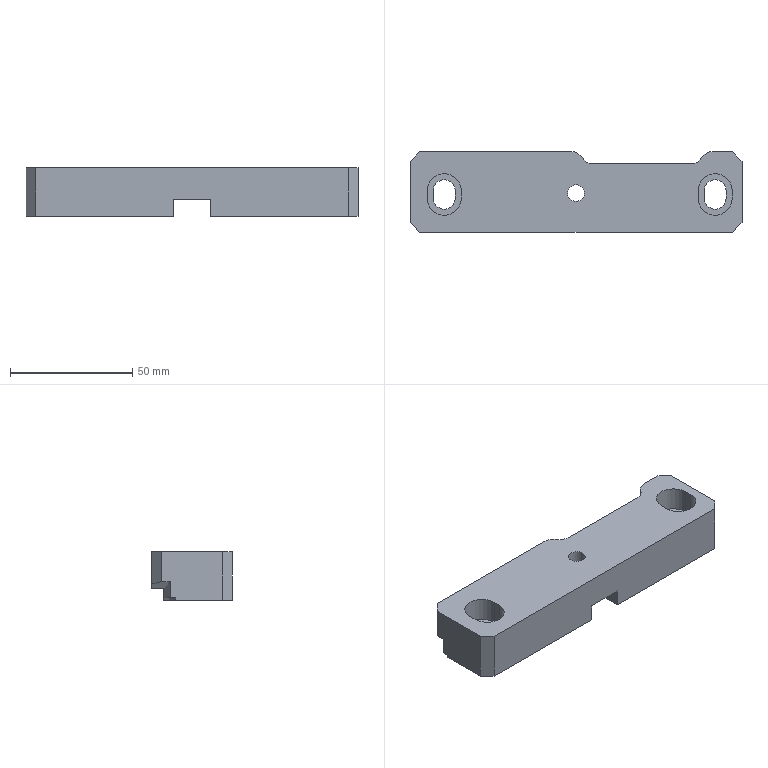Part | NX | features 20 2 | 1 solid | 49 faces | box 136 x 33 x 20 mm | volume 72364 mm3 | plane 35 | cylinder 14 | commonest cylinder face diameters 9 x4 10 x4 14 x4 6.8 x1 24 x1
STEP:
#1=CARTESIAN_POINT('',(810.268,-417.5,16.5));
#2=VERTEX_POINT('',#1);
#3=CARTESIAN_POINT('',(748.002,-417.5,16.5));
#4=VERTEX_POINT('',#3);
#5=CARTESIAN_POINT('',(932.002,-417.5,16.5));
#6=DIRECTION('',(-1.,0.,0.));
#7=VECTOR('',#6,1000.);
#8=LINE('',#5,#7);
#9=EDGE_CURVE('',#2,#4,#8,.T.);
#10=ORIENTED_EDGE('',*,*,#9,.T.);
#11=CARTESIAN_POINT('',(744.002,-421.5,16.5));
#12=VERTEX_POINT('',#11);
#13=CARTESIAN_POINT('',(744.002,-421.5,16.5));
#14=DIRECTION('',(-0.7071,-0.7071,0.));
#15=VECTOR('',#14,1000.);
#16=LINE('',#13,#15);
#17=EDGE_CURVE('',#4,#12,#16,.T.);
#18=ORIENTED_EDGE('',*,*,#17,.T.);
#19=CARTESIAN_POINT('',(744.002,-446.5,16.5));
#20=VERTEX_POINT('',#19);
#21=CARTESIAN_POINT('',(744.002,-417.5,16.5));
#22=DIRECTION('',(0.,-1.,0.));
#23=VECTOR('',#22,1000.);
#24=LINE('',#21,#23);
#25=EDGE_CURVE('',#12,#20,#24,.T.);
#26=ORIENTED_EDGE('',*,*,#25,.T.);
#27=CARTESIAN_POINT('',(748.002,-450.5,16.5));
#28=VERTEX_POINT('',#27);
#29=CARTESIAN_POINT('',(748.002,-450.5,16.5));
#30=DIRECTION('',(0.7071,-0.7071,0.));
#31=VECTOR('',#30,1000.);
#32=LINE('',#29,#31);
#33=EDGE_CURVE('',#20,#28,#32,.T.);
#34=ORIENTED_EDGE('',*,*,#33,.T.);
#35=CARTESIAN_POINT('',(876.002,-450.5,16.5));
#36=VERTEX_POINT('',#35);
#37=CARTESIAN_POINT('',(852.002,-450.5,16.5));
#38=DIRECTION('',(1.,0.,0.));
#39=VECTOR('',#38,1000.);
#40=LINE('',#37,#39);
#41=EDGE_CURVE('',#28,#36,#40,.T.);
#42=ORIENTED_EDGE('',*,*,#41,.T.);
#43=CARTESIAN_POINT('',(880.002,-446.5,16.5));
#44=VERTEX_POINT('',#43);
#45=CARTESIAN_POINT('',(880.002,-446.5,16.5));
#46=DIRECTION('',(0.7071,0.7071,0.));
#47=VECTOR('',#46,1000.);
#48=LINE('',#45,#47);
#49=EDGE_CURVE('',#36,#44,#48,.T.);
#50=ORIENTED_EDGE('',*,*,#49,.T.);
#51=CARTESIAN_POINT('',(880.002,-421.5,16.5));
#52=VERTEX_POINT('',#51);
#53=CARTESIAN_POINT('',(880.002,-450.5,16.5));
#54=DIRECTION('',(0.,1.,0.));
#55=VECTOR('',#54,1000.);
#56=LINE('',#53,#55);
#57=EDGE_CURVE('',#44,#52,#56,.T.);
#58=ORIENTED_EDGE('',*,*,#57,.T.);
#59=CARTESIAN_POINT('',(876.002,-417.5,16.5));
#60=VERTEX_POINT('',#59);
#61=CARTESIAN_POINT('',(876.002,-417.5,16.5));
#62=DIRECTION('',(-0.7071,0.7071,0.));
#63=VECTOR('',#62,1000.);
#64=LINE('',#61,#63);
#65=EDGE_CURVE('',#52,#60,#64,.T.);
#66=ORIENTED_EDGE('',*,*,#65,.T.);
#67=CARTESIAN_POINT('',(867.789,-417.5,16.5));
#68=VERTEX_POINT('',#67);
#69=CARTESIAN_POINT('',(932.002,-417.5,16.5));
#70=DIRECTION('',(-1.,0.,0.));
#71=VECTOR('',#70,1000.);
#72=LINE('',#69,#71);
#73=EDGE_CURVE('',#60,#68,#72,.T.);
#74=ORIENTED_EDGE('',*,*,#73,.T.);
#75=CARTESIAN_POINT('',(863.459,-420.,16.5));
#76=VERTEX_POINT('',#75);
#77=CARTESIAN_POINT('',(867.789,-422.5,16.5));
#78=DIRECTION('',(0.,0.,1.));
#79=DIRECTION('',(1.,0.,0.));
#80=AXIS2_PLACEMENT_3D('',#77,#78,#79);
#81=CIRCLE('',#80,5.);
#82=EDGE_CURVE('',#68,#76,#81,.T.);
#83=ORIENTED_EDGE('',*,*,#82,.T.);
#84=CARTESIAN_POINT('',(859.129,-422.5,16.5));
#85=VERTEX_POINT('',#84);
#86=CARTESIAN_POINT('',(859.129,-417.5,16.5));
#87=DIRECTION('',(0.,0.,1.));
#88=DIRECTION('',(1.,0.,0.));
#89=AXIS2_PLACEMENT_3D('',#86,#87,#88);
#90=CIRCLE('',#89,5.);
#91=EDGE_CURVE('',#85,#76,#90,.T.);
#92=ORIENTED_EDGE('',*,*,#91,.F.);
#93=CARTESIAN_POINT('',(818.929,-422.5,16.5));
#94=VERTEX_POINT('',#93);
#95=CARTESIAN_POINT('',(932.002,-422.5,16.5));
#96=DIRECTION('',(1.,0.,0.));
#97=VECTOR('',#96,1000.);
#98=LINE('',#95,#97);
#99=EDGE_CURVE('',#94,#85,#98,.T.);
#100=ORIENTED_EDGE('',*,*,#99,.F.);
#101=CARTESIAN_POINT('',(814.598,-420.,16.5));
#102=VERTEX_POINT('',#101);
#103=CARTESIAN_POINT('',(818.929,-417.5,16.5));
#104=DIRECTION('',(0.,0.,1.));
#105=DIRECTION('',(1.,0.,0.));
#106=AXIS2_PLACEMENT_3D('',#103,#104,#105);
#107=CIRCLE('',#106,5.);
#108=EDGE_CURVE('',#102,#94,#107,.T.);
#109=ORIENTED_EDGE('',*,*,#108,.F.);
#110=CARTESIAN_POINT('',(810.268,-422.5,16.5));
#111=DIRECTION('',(0.,0.,1.));
#112=DIRECTION('',(1.,0.,0.));
#113=AXIS2_PLACEMENT_3D('',#110,#111,#112);
#114=CIRCLE('',#113,5.);
#115=EDGE_CURVE('',#102,#2,#114,.T.);
#116=ORIENTED_EDGE('',*,*,#115,.T.);
#117=EDGE_LOOP('',(#10,#18,#26,#34,#42,#50,#58,#66,#74,#83,#92,#100,#109,#116));
#118=FACE_BOUND('',#117,.T.);
#119=CARTESIAN_POINT('',(751.002,-433.5,16.5));
#120=VERTEX_POINT('',#119);
#121=CARTESIAN_POINT('',(751.002,-436.5,16.5));
#122=VERTEX_POINT('',#121);
#123=CARTESIAN_POINT('',(751.002,-450.5,16.5));
#124=DIRECTION('',(0.,-1.,0.));
#125=VECTOR('',#124,1000.);
#126=LINE('',#123,#125);
#127=EDGE_CURVE('',#120,#122,#126,.T.);
#128=ORIENTED_EDGE('',*,*,#127,.F.);
#129=CARTESIAN_POINT('',(765.002,-433.5,16.5));
#130=VERTEX_POINT('',#129);
#131=CARTESIAN_POINT('',(758.002,-433.5,16.5));
#132=DIRECTION('',(0.,0.,1.));
#133=DIRECTION('',(1.,0.,0.));
#134=AXIS2_PLACEMENT_3D('',#131,#132,#133);
#135=CIRCLE('',#134,7.);
#136=EDGE_CURVE('',#130,#120,#135,.T.);
#137=ORIENTED_EDGE('',*,*,#136,.F.);
#138=CARTESIAN_POINT('',(765.002,-436.5,16.5));
#139=VERTEX_POINT('',#138);
#140=CARTESIAN_POINT('',(765.002,-450.5,16.5));
#141=DIRECTION('',(0.,1.,0.));
#142=VECTOR('',#141,1000.);
#143=LINE('',#140,#142);
#144=EDGE_CURVE('',#139,#130,#143,.T.);
#145=ORIENTED_EDGE('',*,*,#144,.F.);
#146=CARTESIAN_POINT('',(758.002,-436.5,16.5));
#147=DIRECTION('',(0.,0.,1.));
#148=DIRECTION('',(1.,0.,0.));
#149=AXIS2_PLACEMENT_3D('',#146,#147,#148);
#150=CIRCLE('',#149,7.);
#151=EDGE_CURVE('',#122,#139,#150,.T.);
#152=ORIENTED_EDGE('',*,*,#151,.F.);
#153=EDGE_LOOP('',(#128,#137,#145,#152));
#154=FACE_BOUND('',#153,.T.);
#155=CARTESIAN_POINT('',(862.002,-433.5,16.5));
#156=VERTEX_POINT('',#155);
#157=CARTESIAN_POINT('',(862.002,-436.5,16.5));
#158=VERTEX_POINT('',#157);
#159=CARTESIAN_POINT('',(862.002,-450.5,16.5));
#160=DIRECTION('',(0.,-1.,0.));
#161=VECTOR('',#160,1000.);
#162=LINE('',#159,#161);
#163=EDGE_CURVE('',#156,#158,#162,.T.);
#164=ORIENTED_EDGE('',*,*,#163,.F.);
#165=CARTESIAN_POINT('',(876.002,-433.5,16.5));
#166=VERTEX_POINT('',#165);
#167=CARTESIAN_POINT('',(869.002,-433.5,16.5));
#168=DIRECTION('',(0.,0.,1.));
#169=DIRECTION('',(1.,0.,0.));
#170=AXIS2_PLACEMENT_3D('',#167,#168,#169);
#171=CIRCLE('',#170,7.);
#172=EDGE_CURVE('',#166,#156,#171,.T.);
#173=ORIENTED_EDGE('',*,*,#172,.F.);
#174=CARTESIAN_POINT('',(876.002,-436.5,16.5));
#175=VERTEX_POINT('',#174);
#176=CARTESIAN_POINT('',(876.002,-450.5,16.5));
#177=DIRECTION('',(0.,1.,0.));
#178=VECTOR('',#177,1000.);
#179=LINE('',#176,#178);
#180=EDGE_CURVE('',#175,#166,#179,.T.);
#181=ORIENTED_EDGE('',*,*,#180,.F.);
#182=CARTESIAN_POINT('',(869.002,-436.5,16.5));
#183=DIRECTION('',(0.,0.,1.));
#184=DIRECTION('',(1.,0.,0.));
#185=AXIS2_PLACEMENT_3D('',#182,#183,#184);
#186=CIRCLE('',#185,7.);
#187=EDGE_CURVE('',#158,#175,#186,.T.);
#188=ORIENTED_EDGE('',*,*,#187,.F.);
#189=EDGE_LOOP('',(#164,#173,#181,#188));
#190=FACE_BOUND('',#189,.T.);
#191=CARTESIAN_POINT('',(815.402,-434.5,16.5));
#192=VERTEX_POINT('',#191);
#193=CARTESIAN_POINT('',(812.002,-434.5,16.5));
#194=DIRECTION('',(0.,0.,-1.));
#195=DIRECTION('',(1.,0.,0.));
#196=AXIS2_PLACEMENT_3D('',#193,#194,#195);
#197=CIRCLE('',#196,3.4);
#198=EDGE_CURVE('',#192,#192,#197,.T.);
#199=ORIENTED_EDGE('',*,*,#198,.T.);
#200=EDGE_LOOP('',(#199));
#201=FACE_BOUND('',#200,.T.);
#202=CARTESIAN_POINT('',(932.002,-450.5,16.5));
#203=DIRECTION('',(0.,0.,1.));
#204=DIRECTION('',(-1.,0.,0.));
#205=AXIS2_PLACEMENT_3D('',#202,#203,#204);
#206=PLANE('',#205);
#207=ADVANCED_FACE('',(#118,#154,#190,#201),#206,.T.);
#208=CARTESIAN_POINT('',(754.002,-417.5,1.5));
#209=VERTEX_POINT('',#208);
#210=CARTESIAN_POINT('',(804.502,-417.5,1.5));
#211=VERTEX_POINT('',#210);
#212=CARTESIAN_POINT('',(880.002,-417.5,1.5));
#213=DIRECTION('',(1.,0.,0.));
#214=VECTOR('',#213,1000.);
#215=LINE('',#212,#214);
#216=EDGE_CURVE('',#209,#211,#215,.T.);
#217=ORIENTED_EDGE('',*,*,#216,.T.);
#218=CARTESIAN_POINT('',(804.502,-422.5,1.5));
#219=VERTEX_POINT('',#218);
#220=CARTESIAN_POINT('',(804.502,-396.891,1.5));
#221=DIRECTION('',(0.,-1.,0.));
#222=VECTOR('',#221,1000.);
#223=LINE('',#220,#222);
#224=EDGE_CURVE('',#211,#219,#223,.T.);
#225=ORIENTED_EDGE('',*,*,#224,.T.);
#226=CARTESIAN_POINT('',(754.002,-422.5,1.5));
#227=VERTEX_POINT('',#226);
#228=CARTESIAN_POINT('',(870.001,-422.5,1.5));
#229=DIRECTION('',(1.,0.,0.));
#230=VECTOR('',#229,1000.);
#231=LINE('',#228,#230);
#232=EDGE_CURVE('',#227,#219,#231,.T.);
#233=ORIENTED_EDGE('',*,*,#232,.F.);
#234=CARTESIAN_POINT('',(754.002,-417.5,1.5));
#235=DIRECTION('',(0.,1.,0.));
#236=VECTOR('',#235,1000.);
#237=LINE('',#234,#236);
#238=EDGE_CURVE('',#227,#209,#237,.T.);
#239=ORIENTED_EDGE('',*,*,#238,.T.);
#240=EDGE_LOOP('',(#217,#225,#233,#239));
#241=FACE_BOUND('',#240,.T.);
#242=CARTESIAN_POINT('',(902.273,-396.891,1.5));
#243=DIRECTION('',(0.,0.,-1.));
#244=DIRECTION('',(1.,0.,0.));
#245=AXIS2_PLACEMENT_3D('',#242,#243,#244);
#246=PLANE('',#245);
#247=ADVANCED_FACE('',(#241),#246,.T.);
#248=CARTESIAN_POINT('',(804.502,-422.5,-3.5));
#249=VERTEX_POINT('',#248);
#250=CARTESIAN_POINT('',(804.502,-422.5,3.5));
#251=DIRECTION('',(0.,0.,1.));
#252=VECTOR('',#251,1000.);
#253=LINE('',#250,#252);
#254=EDGE_CURVE('',#249,#219,#253,.T.);
#255=ORIENTED_EDGE('',*,*,#254,.F.);
#256=CARTESIAN_POINT('',(800.711,-422.5,-3.5));
#257=VERTEX_POINT('',#256);
#258=CARTESIAN_POINT('',(838.001,-422.5,-3.5));
#259=DIRECTION('',(-1.,0.,0.));
#260=VECTOR('',#259,1000.);
#261=LINE('',#258,#260);
#262=EDGE_CURVE('',#249,#257,#261,.T.);
#263=ORIENTED_EDGE('',*,*,#262,.T.);
#264=CARTESIAN_POINT('',(800.711,-422.5,-2.5));
#265=VERTEX_POINT('',#264);
#266=CARTESIAN_POINT('',(800.711,-422.5,-2.5));
#267=DIRECTION('',(0.,0.,-1.));
#268=VECTOR('',#267,1000.);
#269=LINE('',#266,#268);
#270=EDGE_CURVE('',#265,#257,#269,.T.);
#271=ORIENTED_EDGE('',*,*,#270,.F.);
#272=CARTESIAN_POINT('',(754.001,-422.5,-2.5));
#273=VERTEX_POINT('',#272);
#274=CARTESIAN_POINT('',(870.001,-422.5,-2.5));
#275=DIRECTION('',(-1.,0.,0.));
#276=VECTOR('',#275,1000.);
#277=LINE('',#274,#276);
#278=EDGE_CURVE('',#265,#273,#277,.T.);
#279=ORIENTED_EDGE('',*,*,#278,.T.);
#280=CARTESIAN_POINT('',(754.001,-422.5,1.5));
#281=VERTEX_POINT('',#280);
#282=CARTESIAN_POINT('',(754.001,-422.5,3.5));
#283=DIRECTION('',(0.,0.,1.));
#284=VECTOR('',#283,1000.);
#285=LINE('',#282,#284);
#286=EDGE_CURVE('',#273,#281,#285,.T.);
#287=ORIENTED_EDGE('',*,*,#286,.T.);
#288=CARTESIAN_POINT('',(754.002,-422.5,1.5));
#289=DIRECTION('',(0.9659,0.,-0.2588));
#290=VECTOR('',#289,1000.);
#291=LINE('',#288,#290);
#292=EDGE_CURVE('',#281,#227,#291,.T.);
#293=ORIENTED_EDGE('',*,*,#292,.T.);
#294=ORIENTED_EDGE('',*,*,#232,.T.);
#295=EDGE_LOOP('',(#255,#263,#271,#279,#287,#293,#294));
#296=FACE_BOUND('',#295,.T.);
#297=CARTESIAN_POINT('',(838.001,-422.5,3.5));
#298=DIRECTION('',(0.,-1.,0.));
#299=DIRECTION('',(0.,0.,1.));
#300=AXIS2_PLACEMENT_3D('',#297,#298,#299);
#301=PLANE('',#300);
#302=ADVANCED_FACE('',(#296),#301,.F.);
#303=CARTESIAN_POINT('',(762.502,-433.5,-3.5));
#304=VERTEX_POINT('',#303);
#305=CARTESIAN_POINT('',(762.502,-436.5,-3.5));
#306=VERTEX_POINT('',#305);
#307=CARTESIAN_POINT('',(762.502,-450.5,-3.5));
#308=DIRECTION('',(0.,-1.,0.));
#309=VECTOR('',#308,1000.);
#310=LINE('',#307,#309);
#311=EDGE_CURVE('',#304,#306,#310,.T.);
#312=ORIENTED_EDGE('',*,*,#311,.F.);
#313=CARTESIAN_POINT('',(753.502,-433.5,-3.5));
#314=VERTEX_POINT('',#313);
#315=CARTESIAN_POINT('',(758.002,-433.5,-3.5));
#316=DIRECTION('',(0.,0.,-1.));
#317=DIRECTION('',(1.,0.,0.));
#318=AXIS2_PLACEMENT_3D('',#315,#316,#317);
#319=CIRCLE('',#318,4.5);
#320=EDGE_CURVE('',#314,#304,#319,.T.);
#321=ORIENTED_EDGE('',*,*,#320,.F.);
#322=CARTESIAN_POINT('',(753.502,-436.5,-3.5));
#323=VERTEX_POINT('',#322);
#324=CARTESIAN_POINT('',(753.502,-450.5,-3.5));
#325=DIRECTION('',(0.,1.,0.));
#326=VECTOR('',#325,1000.);
#327=LINE('',#324,#326);
#328=EDGE_CURVE('',#323,#314,#327,.T.);
#329=ORIENTED_EDGE('',*,*,#328,.F.);
#330=CARTESIAN_POINT('',(758.002,-436.5,-3.5));
#331=DIRECTION('',(0.,0.,-1.));
#332=DIRECTION('',(1.,0.,0.));
#333=AXIS2_PLACEMENT_3D('',#330,#331,#332);
#334=CIRCLE('',#333,4.5);
#335=EDGE_CURVE('',#306,#323,#334,.T.);
#336=ORIENTED_EDGE('',*,*,#335,.F.);
#337=EDGE_LOOP('',(#312,#321,#329,#336));
#338=FACE_BOUND('',#337,.T.);
#339=CARTESIAN_POINT('',(804.502,-450.5,-3.5));
#340=VERTEX_POINT('',#339);
#341=CARTESIAN_POINT('',(804.502,-450.5,-3.5));
#342=DIRECTION('',(0.,1.,0.));
#343=VECTOR('',#342,1000.);
#344=LINE('',#341,#343);
#345=EDGE_CURVE('',#340,#249,#344,.T.);
#346=ORIENTED_EDGE('',*,*,#345,.F.);
#347=CARTESIAN_POINT('',(748.002,-450.5,-3.5));
#348=VERTEX_POINT('',#347);
#349=CARTESIAN_POINT('',(862.002,-450.5,-3.5));
#350=DIRECTION('',(1.,0.,0.));
#351=VECTOR('',#350,1000.);
#352=LINE('',#349,#351);
#353=EDGE_CURVE('',#348,#340,#352,.T.);
#354=ORIENTED_EDGE('',*,*,#353,.F.);
#355=CARTESIAN_POINT('',(744.002,-446.5,-3.5));
#356=VERTEX_POINT('',#355);
#357=CARTESIAN_POINT('',(748.002,-450.5,-3.5));
#358=DIRECTION('',(-0.7071,0.7071,0.));
#359=VECTOR('',#358,1000.);
#360=LINE('',#357,#359);
#361=EDGE_CURVE('',#348,#356,#360,.T.);
#362=ORIENTED_EDGE('',*,*,#361,.T.);
#363=CARTESIAN_POINT('',(744.002,-427.372,-3.5));
#364=VERTEX_POINT('',#363);
#365=CARTESIAN_POINT('',(744.002,-417.5,-3.5));
#366=DIRECTION('',(0.,-1.,0.));
#367=VECTOR('',#366,1000.);
#368=LINE('',#365,#367);
#369=EDGE_CURVE('',#364,#356,#368,.T.);
#370=ORIENTED_EDGE('',*,*,#369,.F.);
#371=CARTESIAN_POINT('',(791.057,-427.372,-3.5));
#372=VERTEX_POINT('',#371);
#373=CARTESIAN_POINT('',(932.002,-427.372,-3.5));
#374=DIRECTION('',(1.,0.,0.));
#375=VECTOR('',#374,1000.);
#376=LINE('',#373,#375);
#377=EDGE_CURVE('',#364,#372,#376,.T.);
#378=ORIENTED_EDGE('',*,*,#377,.T.);
#379=CARTESIAN_POINT('',(791.057,-415.372,-3.5));
#380=DIRECTION('',(0.,0.,-1.));
#381=DIRECTION('',(1.,0.,0.));
#382=AXIS2_PLACEMENT_3D('',#379,#380,#381);
#383=CIRCLE('',#382,12.);
#384=EDGE_CURVE('',#257,#372,#383,.T.);
#385=ORIENTED_EDGE('',*,*,#384,.F.);
#386=ORIENTED_EDGE('',*,*,#262,.F.);
#387=EDGE_LOOP('',(#346,#354,#362,#370,#378,#385,#386));
#388=FACE_BOUND('',#387,.T.);
#389=CARTESIAN_POINT('',(932.002,-450.5,-3.5));
#390=DIRECTION('',(0.,0.,1.));
#391=DIRECTION('',(-1.,0.,0.));
#392=AXIS2_PLACEMENT_3D('',#389,#390,#391);
#393=PLANE('',#392);
#394=ADVANCED_FACE('',(#338,#388),#393,.F.);
#395=CARTESIAN_POINT('',(791.057,-427.372,-2.5));
#396=VERTEX_POINT('',#395);
#397=CARTESIAN_POINT('',(791.057,-427.372,-43.5));
#398=DIRECTION('',(0.,0.,1.));
#399=VECTOR('',#398,1000.);
#400=LINE('',#397,#399);
#401=EDGE_CURVE('',#372,#396,#400,.T.);
#402=ORIENTED_EDGE('',*,*,#401,.T.);
#403=CARTESIAN_POINT('',(791.057,-415.372,-2.5));
#404=DIRECTION('',(0.,0.,1.));
#405=DIRECTION('',(1.,0.,0.));
#406=AXIS2_PLACEMENT_3D('',#403,#404,#405);
#407=CIRCLE('',#406,12.);
#408=EDGE_CURVE('',#396,#265,#407,.T.);
#409=ORIENTED_EDGE('',*,*,#408,.T.);
#410=ORIENTED_EDGE('',*,*,#270,.T.);
#411=ORIENTED_EDGE('',*,*,#384,.T.);
#412=EDGE_LOOP('',(#402,#409,#410,#411));
#413=FACE_BOUND('',#412,.T.);
#414=CARTESIAN_POINT('',(791.057,-415.372,-43.5));
#415=DIRECTION('',(0.,0.,1.));
#416=DIRECTION('',(-1.,0.,0.));
#417=AXIS2_PLACEMENT_3D('',#414,#415,#416);
#418=CYLINDRICAL_SURFACE('',#417,12.);
#419=ADVANCED_FACE('',(#413),#418,.F.);
#420=ORIENTED_EDGE('',*,*,#25,.F.);
#421=CARTESIAN_POINT('',(744.002,-421.5,4.179));
#422=VERTEX_POINT('',#421);
#423=CARTESIAN_POINT('',(744.002,-421.5,11.5));
#424=DIRECTION('',(0.,0.,-1.));
#425=VECTOR('',#424,1000.);
#426=LINE('',#423,#425);
#427=EDGE_CURVE('',#12,#422,#426,.T.);
#428=ORIENTED_EDGE('',*,*,#427,.T.);
#429=CARTESIAN_POINT('',(744.002,-425.179,4.179));
#430=VERTEX_POINT('',#429);
#431=CARTESIAN_POINT('',(744.002,-425.179,4.179));
#432=DIRECTION('',(0.,-1.,0.));
#433=VECTOR('',#432,1000.);
#434=LINE('',#431,#433);
#435=EDGE_CURVE('',#422,#430,#434,.T.);
#436=ORIENTED_EDGE('',*,*,#435,.T.);
#437=CARTESIAN_POINT('',(744.002,-425.179,-2.5));
#438=VERTEX_POINT('',#437);
#439=CARTESIAN_POINT('',(744.002,-425.179,3.5));
#440=DIRECTION('',(0.,0.,-1.));
#441=VECTOR('',#440,1000.);
#442=LINE('',#439,#441);
#443=EDGE_CURVE('',#430,#438,#442,.T.);
#444=ORIENTED_EDGE('',*,*,#443,.T.);
#445=CARTESIAN_POINT('',(744.002,-427.372,-2.5));
#446=VERTEX_POINT('',#445);
#447=CARTESIAN_POINT('',(744.002,-417.5,-2.5));
#448=DIRECTION('',(0.,-1.,0.));
#449=VECTOR('',#448,1000.);
#450=LINE('',#447,#449);
#451=EDGE_CURVE('',#438,#446,#450,.T.);
#452=ORIENTED_EDGE('',*,*,#451,.T.);
#453=CARTESIAN_POINT('',(744.002,-427.372,11.5));
#454=DIRECTION('',(0.,0.,1.));
#455=VECTOR('',#454,1000.);
#456=LINE('',#453,#455);
#457=EDGE_CURVE('',#364,#446,#456,.T.);
#458=ORIENTED_EDGE('',*,*,#457,.F.);
#459=ORIENTED_EDGE('',*,*,#369,.T.);
#460=CARTESIAN_POINT('',(744.002,-446.5,11.5));
#461=DIRECTION('',(0.,0.,1.));
#462=VECTOR('',#461,1000.);
#463=LINE('',#460,#462);
#464=EDGE_CURVE('',#356,#20,#463,.T.);
#465=ORIENTED_EDGE('',*,*,#464,.T.);
#466=EDGE_LOOP('',(#420,#428,#436,#444,#452,#458,#459,#465));
#467=FACE_BOUND('',#466,.T.);
#468=CARTESIAN_POINT('',(744.002,-417.5,11.5));
#469=DIRECTION('',(1.,0.,0.));
#470=DIRECTION('',(0.,0.,1.));
#471=AXIS2_PLACEMENT_3D('',#468,#469,#470);
#472=PLANE('',#471);
#473=ADVANCED_FACE('',(#467),#472,.F.);
#474=ORIENTED_EDGE('',*,*,#451,.F.);
#475=CARTESIAN_POINT('',(754.001,-422.5,-2.5));
#476=DIRECTION('',(-0.9659,-0.2588,0.));
#477=VECTOR('',#476,1000.);
#478=LINE('',#475,#477);
#479=EDGE_CURVE('',#273,#438,#478,.T.);
#480=ORIENTED_EDGE('',*,*,#479,.F.);
#481=ORIENTED_EDGE('',*,*,#278,.F.);
#482=ORIENTED_EDGE('',*,*,#408,.F.);
#483=CARTESIAN_POINT('',(932.002,-427.372,-2.5));
#484=DIRECTION('',(-1.,0.,0.));
#485=VECTOR('',#484,1000.);
#486=LINE('',#483,#485);
#487=EDGE_CURVE('',#396,#446,#486,.T.);
#488=ORIENTED_EDGE('',*,*,#487,.T.);
#489=EDGE_LOOP('',(#474,#480,#481,#482,#488));
#490=FACE_BOUND('',#489,.T.);
#491=CARTESIAN_POINT('',(932.002,-450.5,-2.5));
#492=DIRECTION('',(0.,0.,1.));
#493=DIRECTION('',(-1.,0.,0.));
#494=AXIS2_PLACEMENT_3D('',#491,#492,#493);
#495=PLANE('',#494);
#496=ADVANCED_FACE('',(#490),#495,.F.);
#497=CARTESIAN_POINT('',(810.268,-417.5,3.5));
#498=VERTEX_POINT('',#497);
#499=CARTESIAN_POINT('',(810.268,-417.5,11.5));
#500=DIRECTION('',(0.,0.,-1.));
#501=VECTOR('',#500,1000.);
#502=LINE('',#499,#501);
#503=EDGE_CURVE('',#2,#498,#502,.T.);
#504=ORIENTED_EDGE('',*,*,#503,.T.);
#505=CARTESIAN_POINT('',(804.502,-417.5,3.5));
#506=VERTEX_POINT('',#505);
#507=CARTESIAN_POINT('',(962.502,-417.5,3.5));
#508=DIRECTION('',(-1.,0.,0.));
#509=VECTOR('',#508,1000.);
#510=LINE('',#507,#509);
#511=EDGE_CURVE('',#498,#506,#510,.T.);
#512=ORIENTED_EDGE('',*,*,#511,.T.);
#513=CARTESIAN_POINT('',(804.502,-417.5,-16.5));
#514=DIRECTION('',(0.,0.,1.));
#515=VECTOR('',#514,1000.);
#516=LINE('',#513,#515);
#517=EDGE_CURVE('',#211,#506,#516,.T.);
#518=ORIENTED_EDGE('',*,*,#517,.F.);
#519=ORIENTED_EDGE('',*,*,#216,.F.);
#520=CARTESIAN_POINT('',(748.002,-417.5,3.108));
#521=VERTEX_POINT('',#520);
#522=CARTESIAN_POINT('',(754.002,-417.5,1.5));
#523=DIRECTION('',(-0.9659,0.,0.2588));
#524=VECTOR('',#523,1000.);
#525=LINE('',#522,#524);
#526=EDGE_CURVE('',#209,#521,#525,.T.);
#527=ORIENTED_EDGE('',*,*,#526,.T.);
#528=CARTESIAN_POINT('',(748.002,-417.5,11.5));
#529=DIRECTION('',(0.,0.,1.));
#530=VECTOR('',#529,1000.);
#531=LINE('',#528,#530);
#532=EDGE_CURVE('',#521,#4,#531,.T.);
#533=ORIENTED_EDGE('',*,*,#532,.T.);
#534=ORIENTED_EDGE('',*,*,#9,.F.);
#535=EDGE_LOOP('',(#504,#512,#518,#519,#527,#533,#534));
#536=FACE_BOUND('',#535,.T.);
#537=CARTESIAN_POINT('',(932.002,-417.5,11.5));
#538=DIRECTION('',(0.,-1.,0.));
#539=DIRECTION('',(0.,0.,1.));
#540=AXIS2_PLACEMENT_3D('',#537,#538,#539);
#541=PLANE('',#540);
#542=ADVANCED_FACE('',(#536),#541,.F.);
#543=CARTESIAN_POINT('',(870.001,-422.5,-3.5));
#544=VERTEX_POINT('',#543);
#545=CARTESIAN_POINT('',(819.502,-422.5,-3.5));
#546=VERTEX_POINT('',#545);
#547=CARTESIAN_POINT('',(838.001,-422.5,-3.5));
#548=DIRECTION('',(-1.,0.,0.));
#549=VECTOR('',#548,1000.);
#550=LINE('',#547,#549);
#551=EDGE_CURVE('',#544,#546,#550,.T.);
#552=ORIENTED_EDGE('',*,*,#551,.T.);
#553=CARTESIAN_POINT('',(819.502,-422.5,3.5));
#554=VERTEX_POINT('',#553);
#555=CARTESIAN_POINT('',(819.502,-422.5,3.5));
#556=DIRECTION('',(0.,0.,1.));
#557=VECTOR('',#556,1000.);
#558=LINE('',#555,#557);
#559=EDGE_CURVE('',#546,#554,#558,.T.);
#560=ORIENTED_EDGE('',*,*,#559,.T.);
#561=CARTESIAN_POINT('',(818.929,-422.5,3.5));
#562=VERTEX_POINT('',#561);
#563=CARTESIAN_POINT('',(838.001,-422.5,3.5));
#564=DIRECTION('',(-1.,0.,0.));
#565=VECTOR('',#564,1000.);
#566=LINE('',#563,#565);
#567=EDGE_CURVE('',#554,#562,#566,.T.);
#568=ORIENTED_EDGE('',*,*,#567,.T.);
#569=CARTESIAN_POINT('',(818.929,-422.5,3.5));
#570=DIRECTION('',(0.,0.,-1.));
#571=VECTOR('',#570,1000.);
#572=LINE('',#569,#571);
#573=EDGE_CURVE('',#94,#562,#572,.T.);
#574=ORIENTED_EDGE('',*,*,#573,.F.);
#575=ORIENTED_EDGE('',*,*,#99,.T.);
#576=CARTESIAN_POINT('',(859.129,-422.5,1.5));
#577=VERTEX_POINT('',#576);
#578=CARTESIAN_POINT('',(859.129,-422.5,3.5));
#579=DIRECTION('',(0.,0.,1.));
#580=VECTOR('',#579,1000.);
#581=LINE('',#578,#580);
#582=EDGE_CURVE('',#577,#85,#581,.T.);
#583=ORIENTED_EDGE('',*,*,#582,.F.);
#584=CARTESIAN_POINT('',(870.001,-422.5,1.5));
#585=VERTEX_POINT('',#584);
#586=CARTESIAN_POINT('',(820.273,-422.5,1.5));
#587=DIRECTION('',(1.,0.,0.));
#588=VECTOR('',#587,1000.);
#589=LINE('',#586,#588);
#590=EDGE_CURVE('',#577,#585,#589,.T.);
#591=ORIENTED_EDGE('',*,*,#590,.T.);
#592=CARTESIAN_POINT('',(870.001,-422.5,3.5));
#593=DIRECTION('',(0.,0.,1.));
#594=VECTOR('',#593,1000.);
#595=LINE('',#592,#594);
#596=EDGE_CURVE('',#544,#585,#595,.T.);
#597=ORIENTED_EDGE('',*,*,#596,.F.);
#598=EDGE_LOOP('',(#552,#560,#568,#574,#575,#583,#591,#597));
#599=FACE_BOUND('',#598,.T.);
#600=CARTESIAN_POINT('',(838.001,-422.5,3.5));
#601=DIRECTION('',(0.,-1.,0.));
#602=DIRECTION('',(0.,0.,1.));
#603=AXIS2_PLACEMENT_3D('',#600,#601,#602);
#604=PLANE('',#603);
#605=ADVANCED_FACE('',(#599),#604,.F.);
#606=CARTESIAN_POINT('',(819.502,-450.5,-3.5));
#607=VERTEX_POINT('',#606);
#608=CARTESIAN_POINT('',(876.002,-450.5,-3.5));
#609=VERTEX_POINT('',#608);
#610=CARTESIAN_POINT('',(862.002,-450.5,-3.5));
#611=DIRECTION('',(1.,0.,0.));
#612=VECTOR('',#611,1000.);
#613=LINE('',#610,#612);
#614=EDGE_CURVE('',#607,#609,#613,.T.);
#615=ORIENTED_EDGE('',*,*,#614,.F.);
#616=CARTESIAN_POINT('',(819.502,-450.5,-3.5));
#617=DIRECTION('',(0.,1.,0.));
#618=VECTOR('',#617,1000.);
#619=LINE('',#616,#618);
#620=EDGE_CURVE('',#607,#546,#619,.T.);
#621=ORIENTED_EDGE('',*,*,#620,.T.);
#622=ORIENTED_EDGE('',*,*,#551,.F.);
#623=CARTESIAN_POINT('',(880.002,-425.18,-3.5));
#624=VERTEX_POINT('',#623);
#625=CARTESIAN_POINT('',(880.002,-425.18,-3.5));
#626=DIRECTION('',(-0.9659,0.2588,0.));
#627=VECTOR('',#626,1000.);
#628=LINE('',#625,#627);
#629=EDGE_CURVE('',#624,#544,#628,.T.);
#630=ORIENTED_EDGE('',*,*,#629,.F.);
#631=CARTESIAN_POINT('',(880.002,-446.5,-3.5));
#632=VERTEX_POINT('',#631);
#633=CARTESIAN_POINT('',(880.002,-450.5,-3.5));
#634=DIRECTION('',(0.,1.,0.));
#635=VECTOR('',#634,1000.);
#636=LINE('',#633,#635);
#637=EDGE_CURVE('',#632,#624,#636,.T.);
#638=ORIENTED_EDGE('',*,*,#637,.F.);
#639=CARTESIAN_POINT('',(880.002,-446.5,-3.5));
#640=DIRECTION('',(-0.7071,-0.7071,0.));
#641=VECTOR('',#640,1000.);
#642=LINE('',#639,#641);
#643=EDGE_CURVE('',#632,#609,#642,.T.);
#644=ORIENTED_EDGE('',*,*,#643,.T.);
#645=EDGE_LOOP('',(#615,#621,#622,#630,#638,#644));
#646=FACE_BOUND('',#645,.T.);
#647=CARTESIAN_POINT('',(864.502,-433.5,-3.5));
#648=VERTEX_POINT('',#647);
#649=CARTESIAN_POINT('',(864.502,-436.5,-3.5));
#650=VERTEX_POINT('',#649);
#651=CARTESIAN_POINT('',(864.502,-432.5,-3.5));
#652=DIRECTION('',(0.,-1.,0.));
#653=VECTOR('',#652,1000.);
#654=LINE('',#651,#653);
#655=EDGE_CURVE('',#648,#650,#654,.T.);
#656=ORIENTED_EDGE('',*,*,#655,.T.);
#657=CARTESIAN_POINT('',(873.502,-436.5,-3.5));
#658=VERTEX_POINT('',#657);
#659=CARTESIAN_POINT('',(869.002,-436.5,-3.5));
#660=DIRECTION('',(0.,0.,1.));
#661=DIRECTION('',(1.,0.,0.));
#662=AXIS2_PLACEMENT_3D('',#659,#660,#661);
#663=CIRCLE('',#662,4.5);
#664=EDGE_CURVE('',#650,#658,#663,.T.);
#665=ORIENTED_EDGE('',*,*,#664,.T.);
#666=CARTESIAN_POINT('',(873.502,-433.5,-3.5));
#667=VERTEX_POINT('',#666);
#668=CARTESIAN_POINT('',(873.502,-439.5,-3.5));
#669=DIRECTION('',(0.,1.,0.));
#670=VECTOR('',#669,1000.);
#671=LINE('',#668,#670);
#672=EDGE_CURVE('',#658,#667,#671,.T.);
#673=ORIENTED_EDGE('',*,*,#672,.T.);
#674=CARTESIAN_POINT('',(869.002,-433.5,-3.5));
#675=DIRECTION('',(0.,0.,1.));
#676=DIRECTION('',(1.,0.,0.));
#677=AXIS2_PLACEMENT_3D('',#674,#675,#676);
#678=CIRCLE('',#677,4.5);
#679=EDGE_CURVE('',#667,#648,#678,.T.);
#680=ORIENTED_EDGE('',*,*,#679,.T.);
#681=EDGE_LOOP('',(#656,#665,#673,#680));
#682=FACE_BOUND('',#681,.T.);
#683=CARTESIAN_POINT('',(932.002,-450.5,-3.5));
#684=DIRECTION('',(0.,0.,1.));
#685=DIRECTION('',(-1.,0.,0.));
#686=AXIS2_PLACEMENT_3D('',#683,#684,#685);
#687=PLANE('',#686);
#688=ADVANCED_FACE('',(#646,#682),#687,.F.);
#689=ORIENTED_EDGE('',*,*,#487,.F.);
#690=ORIENTED_EDGE('',*,*,#401,.F.);
#691=ORIENTED_EDGE('',*,*,#377,.F.);
#692=ORIENTED_EDGE('',*,*,#457,.T.);
#693=EDGE_LOOP('',(#689,#690,#691,#692));
#694=FACE_BOUND('',#693,.T.);
#695=CARTESIAN_POINT('',(684.583,-427.372,-21.));
#696=DIRECTION('',(0.,1.,0.));
#697=DIRECTION('',(0.,0.,-1.));
#698=AXIS2_PLACEMENT_3D('',#695,#696,#697);
#699=PLANE('',#698);
#700=ADVANCED_FACE('',(#694),#699,.T.);
#701=ORIENTED_EDGE('',*,*,#643,.F.);
#702=CARTESIAN_POINT('',(880.002,-446.5,11.5));
#703=DIRECTION('',(0.,0.,-1.));
#704=VECTOR('',#703,1000.);
#705=LINE('',#702,#704);
#706=EDGE_CURVE('',#44,#632,#705,.T.);
#707=ORIENTED_EDGE('',*,*,#706,.F.);
#708=ORIENTED_EDGE('',*,*,#49,.F.);
#709=CARTESIAN_POINT('',(876.002,-450.5,11.5));
#710=DIRECTION('',(0.,0.,1.));
#711=VECTOR('',#710,1000.);
#712=LINE('',#709,#711);
#713=EDGE_CURVE('',#609,#36,#712,.T.);
#714=ORIENTED_EDGE('',*,*,#713,.F.);
#715=EDGE_LOOP('',(#701,#707,#708,#714));
#716=FACE_BOUND('',#715,.T.);
#717=CARTESIAN_POINT('',(880.002,-446.5,11.5));
#718=DIRECTION('',(-0.7071,0.7071,0.));
#719=DIRECTION('',(0.,0.,-1.));
#720=AXIS2_PLACEMENT_3D('',#717,#718,#719);
#721=PLANE('',#720);
#722=ADVANCED_FACE('',(#716),#721,.F.);
#723=ORIENTED_EDGE('',*,*,#361,.F.);
#724=CARTESIAN_POINT('',(748.002,-450.5,11.5));
#725=DIRECTION('',(0.,0.,-1.));
#726=VECTOR('',#725,1000.);
#727=LINE('',#724,#726);
#728=EDGE_CURVE('',#28,#348,#727,.T.);
#729=ORIENTED_EDGE('',*,*,#728,.F.);
#730=ORIENTED_EDGE('',*,*,#33,.F.);
#731=ORIENTED_EDGE('',*,*,#464,.F.);
#732=EDGE_LOOP('',(#723,#729,#730,#731));
#733=FACE_BOUND('',#732,.T.);
#734=CARTESIAN_POINT('',(748.002,-450.5,11.5));
#735=DIRECTION('',(0.7071,0.7071,0.));
#736=DIRECTION('',(0.,0.,-1.));
#737=AXIS2_PLACEMENT_3D('',#734,#735,#736);
#738=PLANE('',#737);
#739=ADVANCED_FACE('',(#733),#738,.F.);
#740=ORIENTED_EDGE('',*,*,#187,.T.);
#741=CARTESIAN_POINT('',(876.002,-436.5,6.5));
#742=VERTEX_POINT('',#741);
#743=CARTESIAN_POINT('',(876.002,-436.5,42.5));
#744=DIRECTION('',(0.,0.,1.));
#745=VECTOR('',#744,1000.);
#746=LINE('',#743,#745);
#747=EDGE_CURVE('',#742,#175,#746,.T.);
#748=ORIENTED_EDGE('',*,*,#747,.F.);
#749=CARTESIAN_POINT('',(862.002,-436.5,6.5));
#750=VERTEX_POINT('',#749);
#751=CARTESIAN_POINT('',(869.002,-436.5,6.5));
#752=DIRECTION('',(0.,0.,1.));
#753=DIRECTION('',(-1.,0.,0.));
#754=AXIS2_PLACEMENT_3D('',#751,#752,#753);
#755=CIRCLE('',#754,7.);
#756=EDGE_CURVE('',#750,#742,#755,.T.);
#757=ORIENTED_EDGE('',*,*,#756,.F.);
#758=CARTESIAN_POINT('',(862.002,-436.5,42.5));
#759=DIRECTION('',(0.,0.,1.));
#760=VECTOR('',#759,1000.);
#761=LINE('',#758,#760);
#762=EDGE_CURVE('',#750,#158,#761,.T.);
#763=ORIENTED_EDGE('',*,*,#762,.T.);
#764=EDGE_LOOP('',(#740,#748,#757,#763));
#765=FACE_BOUND('',#764,.T.);
#766=CARTESIAN_POINT('',(869.002,-436.5,42.5));
#767=DIRECTION('',(0.,0.,-1.));
#768=DIRECTION('',(1.,0.,0.));
#769=AXIS2_PLACEMENT_3D('',#766,#767,#768);
#770=CYLINDRICAL_SURFACE('',#769,7.);
#771=ADVANCED_FACE('',(#765),#770,.F.);
#772=CARTESIAN_POINT('',(873.502,-436.5,6.5));
#773=VERTEX_POINT('',#772);
#774=CARTESIAN_POINT('',(864.502,-436.5,6.5));
#775=VERTEX_POINT('',#774);
#776=CARTESIAN_POINT('',(869.002,-436.5,6.5));
#777=DIRECTION('',(0.,0.,-1.));
#778=DIRECTION('',(-1.,0.,0.));
#779=AXIS2_PLACEMENT_3D('',#776,#777,#778);
#780=CIRCLE('',#779,4.5);
#781=EDGE_CURVE('',#773,#775,#780,.T.);
#782=ORIENTED_EDGE('',*,*,#781,.F.);
#783=CARTESIAN_POINT('',(873.502,-436.5,42.5));
#784=DIRECTION('',(0.,0.,1.));
#785=VECTOR('',#784,1000.);
#786=LINE('',#783,#785);
#787=EDGE_CURVE('',#658,#773,#786,.T.);
#788=ORIENTED_EDGE('',*,*,#787,.F.);
#789=ORIENTED_EDGE('',*,*,#664,.F.);
#790=CARTESIAN_POINT('',(864.502,-436.5,42.5));
#791=DIRECTION('',(0.,0.,1.));
#792=VECTOR('',#791,1000.);
#793=LINE('',#790,#792);
#794=EDGE_CURVE('',#650,#775,#793,.T.);
#795=ORIENTED_EDGE('',*,*,#794,.T.);
#796=EDGE_LOOP('',(#782,#788,#789,#795));
#797=FACE_BOUND('',#796,.T.);
#798=CARTESIAN_POINT('',(869.002,-436.5,42.5));
#799=DIRECTION('',(0.,0.,-1.));
#800=DIRECTION('',(1.,0.,0.));
#801=AXIS2_PLACEMENT_3D('',#798,#799,#800);
#802=CYLINDRICAL_SURFACE('',#801,4.5);
#803=ADVANCED_FACE('',(#797),#802,.F.);
#804=CARTESIAN_POINT('',(873.502,-433.5,6.5));
#805=VERTEX_POINT('',#804);
#806=CARTESIAN_POINT('',(873.502,-439.5,6.5));
#807=DIRECTION('',(0.,-1.,0.));
#808=VECTOR('',#807,1000.);
#809=LINE('',#806,#808);
#810=EDGE_CURVE('',#805,#773,#809,.T.);
#811=ORIENTED_EDGE('',*,*,#810,.F.);
#812=CARTESIAN_POINT('',(873.502,-433.5,42.5));
#813=DIRECTION('',(0.,0.,1.));
#814=VECTOR('',#813,1000.);
#815=LINE('',#812,#814);
#816=EDGE_CURVE('',#667,#805,#815,.T.);
#817=ORIENTED_EDGE('',*,*,#816,.F.);
#818=ORIENTED_EDGE('',*,*,#672,.F.);
#819=ORIENTED_EDGE('',*,*,#787,.T.);
#820=EDGE_LOOP('',(#811,#817,#818,#819));
#821=FACE_BOUND('',#820,.T.);
#822=CARTESIAN_POINT('',(873.502,-439.5,42.5));
#823=DIRECTION('',(-1.,0.,0.));
#824=DIRECTION('',(0.,0.,-1.));
#825=AXIS2_PLACEMENT_3D('',#822,#823,#824);
#826=PLANE('',#825);
#827=ADVANCED_FACE('',(#821),#826,.T.);
#828=CARTESIAN_POINT('',(864.502,-433.5,6.5));
#829=VERTEX_POINT('',#828);
#830=CARTESIAN_POINT('',(869.002,-433.5,6.5));
#831=DIRECTION('',(0.,0.,-1.));
#832=DIRECTION('',(-1.,0.,0.));
#833=AXIS2_PLACEMENT_3D('',#830,#831,#832);
#834=CIRCLE('',#833,4.5);
#835=EDGE_CURVE('',#829,#805,#834,.T.);
#836=ORIENTED_EDGE('',*,*,#835,.F.);
#837=CARTESIAN_POINT('',(864.502,-433.5,42.5));
#838=DIRECTION('',(0.,0.,1.));
#839=VECTOR('',#838,1000.);
#840=LINE('',#837,#839);
#841=EDGE_CURVE('',#648,#829,#840,.T.);
#842=ORIENTED_EDGE('',*,*,#841,.F.);
#843=ORIENTED_EDGE('',*,*,#679,.F.);
#844=ORIENTED_EDGE('',*,*,#816,.T.);
#845=EDGE_LOOP('',(#836,#842,#843,#844));
#846=FACE_BOUND('',#845,.T.);
#847=CARTESIAN_POINT('',(869.002,-433.5,42.5));
#848=DIRECTION('',(0.,0.,-1.));
#849=DIRECTION('',(1.,0.,0.));
#850=AXIS2_PLACEMENT_3D('',#847,#848,#849);
#851=CYLINDRICAL_SURFACE('',#850,4.5);
#852=ADVANCED_FACE('',(#846),#851,.F.);
#853=CARTESIAN_POINT('',(864.502,-432.5,6.5));
#854=DIRECTION('',(0.,1.,0.));
#855=VECTOR('',#854,1000.);
#856=LINE('',#853,#855);
#857=EDGE_CURVE('',#775,#829,#856,.T.);
#858=ORIENTED_EDGE('',*,*,#857,.F.);
#859=ORIENTED_EDGE('',*,*,#794,.F.);
#860=ORIENTED_EDGE('',*,*,#655,.F.);
#861=ORIENTED_EDGE('',*,*,#841,.T.);
#862=EDGE_LOOP('',(#858,#859,#860,#861));
#863=FACE_BOUND('',#862,.T.);
#864=CARTESIAN_POINT('',(864.502,-432.5,42.5));
#865=DIRECTION('',(1.,0.,0.));
#866=DIRECTION('',(0.,0.,1.));
#867=AXIS2_PLACEMENT_3D('',#864,#865,#866);
#868=PLANE('',#867);
#869=ADVANCED_FACE('',(#863),#868,.T.);
#870=ORIENTED_EDGE('',*,*,#151,.T.);
#871=CARTESIAN_POINT('',(765.002,-436.5,6.5));
#872=VERTEX_POINT('',#871);
#873=CARTESIAN_POINT('',(765.002,-436.5,42.5));
#874=DIRECTION('',(0.,0.,-1.));
#875=VECTOR('',#874,1000.);
#876=LINE('',#873,#875);
#877=EDGE_CURVE('',#139,#872,#876,.T.);
#878=ORIENTED_EDGE('',*,*,#877,.T.);
#879=CARTESIAN_POINT('',(751.002,-436.5,6.5));
#880=VERTEX_POINT('',#879);
#881=CARTESIAN_POINT('',(758.002,-436.5,6.5));
#882=DIRECTION('',(0.,0.,1.));
#883=DIRECTION('',(-1.,0.,0.));
#884=AXIS2_PLACEMENT_3D('',#881,#882,#883);
#885=CIRCLE('',#884,7.);
#886=EDGE_CURVE('',#880,#872,#885,.T.);
#887=ORIENTED_EDGE('',*,*,#886,.F.);
#888=CARTESIAN_POINT('',(751.002,-436.5,42.5));
#889=DIRECTION('',(0.,0.,-1.));
#890=VECTOR('',#889,1000.);
#891=LINE('',#888,#890);
#892=EDGE_CURVE('',#122,#880,#891,.T.);
#893=ORIENTED_EDGE('',*,*,#892,.F.);
#894=EDGE_LOOP('',(#870,#878,#887,#893));
#895=FACE_BOUND('',#894,.T.);
#896=CARTESIAN_POINT('',(758.002,-436.5,42.5));
#897=DIRECTION('',(0.,0.,-1.));
#898=DIRECTION('',(-1.,0.,0.));
#899=AXIS2_PLACEMENT_3D('',#896,#897,#898);
#900=CYLINDRICAL_SURFACE('',#899,7.);
#901=ADVANCED_FACE('',(#895),#900,.F.);
#902=CARTESIAN_POINT('',(753.502,-433.5,6.5));
#903=VERTEX_POINT('',#902);
#904=CARTESIAN_POINT('',(762.502,-433.5,6.5));
#905=VERTEX_POINT('',#904);
#906=CARTESIAN_POINT('',(758.002,-433.5,6.5));
#907=DIRECTION('',(0.,0.,-1.));
#908=DIRECTION('',(-1.,0.,0.));
#909=AXIS2_PLACEMENT_3D('',#906,#907,#908);
#910=CIRCLE('',#909,4.5);
#911=EDGE_CURVE('',#903,#905,#910,.T.);
#912=ORIENTED_EDGE('',*,*,#911,.F.);
#913=CARTESIAN_POINT('',(753.502,-433.5,42.5));
#914=DIRECTION('',(0.,0.,-1.));
#915=VECTOR('',#914,1000.);
#916=LINE('',#913,#915);
#917=EDGE_CURVE('',#903,#314,#916,.T.);
#918=ORIENTED_EDGE('',*,*,#917,.T.);
#919=ORIENTED_EDGE('',*,*,#320,.T.);
#920=CARTESIAN_POINT('',(762.502,-433.5,42.5));
#921=DIRECTION('',(0.,0.,-1.));
#922=VECTOR('',#921,1000.);
#923=LINE('',#920,#922);
#924=EDGE_CURVE('',#905,#304,#923,.T.);
#925=ORIENTED_EDGE('',*,*,#924,.F.);
#926=EDGE_LOOP('',(#912,#918,#919,#925));
#927=FACE_BOUND('',#926,.T.);
#928=CARTESIAN_POINT('',(758.002,-433.5,42.5));
#929=DIRECTION('',(0.,0.,-1.));
#930=DIRECTION('',(-1.,0.,0.));
#931=AXIS2_PLACEMENT_3D('',#928,#929,#930);
#932=CYLINDRICAL_SURFACE('',#931,4.5);
#933=ADVANCED_FACE('',(#927),#932,.F.);
#934=CARTESIAN_POINT('',(753.502,-436.5,6.5));
#935=VERTEX_POINT('',#934);
#936=CARTESIAN_POINT('',(753.502,-439.5,6.5));
#937=DIRECTION('',(0.,1.,0.));
#938=VECTOR('',#937,1000.);
#939=LINE('',#936,#938);
#940=EDGE_CURVE('',#935,#903,#939,.T.);
#941=ORIENTED_EDGE('',*,*,#940,.F.);
#942=CARTESIAN_POINT('',(753.502,-436.5,42.5));
#943=DIRECTION('',(0.,0.,-1.));
#944=VECTOR('',#943,1000.);
#945=LINE('',#942,#944);
#946=EDGE_CURVE('',#935,#323,#945,.T.);
#947=ORIENTED_EDGE('',*,*,#946,.T.);
#948=ORIENTED_EDGE('',*,*,#328,.T.);
#949=ORIENTED_EDGE('',*,*,#917,.F.);
#950=EDGE_LOOP('',(#941,#947,#948,#949));
#951=FACE_BOUND('',#950,.T.);
#952=CARTESIAN_POINT('',(753.502,-439.5,42.5));
#953=DIRECTION('',(1.,0.,0.));
#954=DIRECTION('',(0.,0.,-1.));
#955=AXIS2_PLACEMENT_3D('',#952,#953,#954);
#956=PLANE('',#955);
#957=ADVANCED_FACE('',(#951),#956,.T.);
#958=CARTESIAN_POINT('',(762.502,-436.5,6.5));
#959=VERTEX_POINT('',#958);
#960=CARTESIAN_POINT('',(758.002,-436.5,6.5));
#961=DIRECTION('',(0.,0.,-1.));
#962=DIRECTION('',(-1.,0.,0.));
#963=AXIS2_PLACEMENT_3D('',#960,#961,#962);
#964=CIRCLE('',#963,4.5);
#965=EDGE_CURVE('',#959,#935,#964,.T.);
#966=ORIENTED_EDGE('',*,*,#965,.F.);
#967=CARTESIAN_POINT('',(762.502,-436.5,42.5));
#968=DIRECTION('',(0.,0.,-1.));
#969=VECTOR('',#968,1000.);
#970=LINE('',#967,#969);
#971=EDGE_CURVE('',#959,#306,#970,.T.);
#972=ORIENTED_EDGE('',*,*,#971,.T.);
#973=ORIENTED_EDGE('',*,*,#335,.T.);
#974=ORIENTED_EDGE('',*,*,#946,.F.);
#975=EDGE_LOOP('',(#966,#972,#973,#974));
#976=FACE_BOUND('',#975,.T.);
#977=CARTESIAN_POINT('',(758.002,-436.5,42.5));
#978=DIRECTION('',(0.,0.,-1.));
#979=DIRECTION('',(-1.,0.,0.));
#980=AXIS2_PLACEMENT_3D('',#977,#978,#979);
#981=CYLINDRICAL_SURFACE('',#980,4.5);
#982=ADVANCED_FACE('',(#976),#981,.F.);
#983=CARTESIAN_POINT('',(762.502,-432.5,6.5));
#984=DIRECTION('',(0.,-1.,0.));
#985=VECTOR('',#984,1000.);
#986=LINE('',#983,#985);
#987=EDGE_CURVE('',#905,#959,#986,.T.);
#988=ORIENTED_EDGE('',*,*,#987,.F.);
#989=ORIENTED_EDGE('',*,*,#924,.T.);
#990=ORIENTED_EDGE('',*,*,#311,.T.);
#991=ORIENTED_EDGE('',*,*,#971,.F.);
#992=EDGE_LOOP('',(#988,#989,#990,#991));
#993=FACE_BOUND('',#992,.T.);
#994=CARTESIAN_POINT('',(762.502,-432.5,42.5));
#995=DIRECTION('',(-1.,0.,0.));
#996=DIRECTION('',(0.,0.,1.));
#997=AXIS2_PLACEMENT_3D('',#994,#995,#996);
#998=PLANE('',#997);
#999=ADVANCED_FACE('',(#993),#998,.T.);
#1000=ORIENTED_EDGE('',*,*,#180,.T.);
#1001=CARTESIAN_POINT('',(876.002,-433.5,6.5));
#1002=VERTEX_POINT('',#1001);
#1003=CARTESIAN_POINT('',(876.002,-433.5,42.5));
#1004=DIRECTION('',(0.,0.,1.));
#1005=VECTOR('',#1004,1000.);
#1006=LINE('',#1003,#1005);
#1007=EDGE_CURVE('',#1002,#166,#1006,.T.);
#1008=ORIENTED_EDGE('',*,*,#1007,.F.);
#1009=CARTESIAN_POINT('',(876.002,-432.5,6.5));
#1010=DIRECTION('',(0.,1.,0.));
#1011=VECTOR('',#1010,1000.);
#1012=LINE('',#1009,#1011);
#1013=EDGE_CURVE('',#742,#1002,#1012,.T.);
#1014=ORIENTED_EDGE('',*,*,#1013,.F.);
#1015=ORIENTED_EDGE('',*,*,#747,.T.);
#1016=EDGE_LOOP('',(#1000,#1008,#1014,#1015));
#1017=FACE_BOUND('',#1016,.T.);
#1018=CARTESIAN_POINT('',(876.002,-432.5,42.5));
#1019=DIRECTION('',(1.,0.,0.));
#1020=DIRECTION('',(0.,0.,1.));
#1021=AXIS2_PLACEMENT_3D('',#1018,#1019,#1020);
#1022=PLANE('',#1021);
#1023=ADVANCED_FACE('',(#1017),#1022,.F.);
#1024=ORIENTED_EDGE('',*,*,#163,.T.);
#1025=ORIENTED_EDGE('',*,*,#762,.F.);
#1026=CARTESIAN_POINT('',(862.002,-433.5,6.5));
#1027=VERTEX_POINT('',#1026);
#1028=CARTESIAN_POINT('',(862.002,-439.5,6.5));
#1029=DIRECTION('',(0.,-1.,0.));
#1030=VECTOR('',#1029,1000.);
#1031=LINE('',#1028,#1030);
#1032=EDGE_CURVE('',#1027,#750,#1031,.T.);
#1033=ORIENTED_EDGE('',*,*,#1032,.F.);
#1034=CARTESIAN_POINT('',(862.002,-433.5,42.5));
#1035=DIRECTION('',(0.,0.,1.));
#1036=VECTOR('',#1035,1000.);
#1037=LINE('',#1034,#1036);
#1038=EDGE_CURVE('',#1027,#156,#1037,.T.);
#1039=ORIENTED_EDGE('',*,*,#1038,.T.);
#1040=EDGE_LOOP('',(#1024,#1025,#1033,#1039));
#1041=FACE_BOUND('',#1040,.T.);
#1042=CARTESIAN_POINT('',(862.002,-439.5,42.5));
#1043=DIRECTION('',(-1.,0.,0.));
#1044=DIRECTION('',(0.,0.,-1.));
#1045=AXIS2_PLACEMENT_3D('',#1042,#1043,#1044);
#1046=PLANE('',#1045);
#1047=ADVANCED_FACE('',(#1041),#1046,.F.);
#1048=ORIENTED_EDGE('',*,*,#144,.T.);
#1049=CARTESIAN_POINT('',(765.002,-433.5,6.5));
#1050=VERTEX_POINT('',#1049);
#1051=CARTESIAN_POINT('',(765.002,-433.5,42.5));
#1052=DIRECTION('',(0.,0.,-1.));
#1053=VECTOR('',#1052,1000.);
#1054=LINE('',#1051,#1053);
#1055=EDGE_CURVE('',#130,#1050,#1054,.T.);
#1056=ORIENTED_EDGE('',*,*,#1055,.T.);
#1057=CARTESIAN_POINT('',(765.002,-439.5,6.5));
#1058=DIRECTION('',(0.,1.,0.));
#1059=VECTOR('',#1058,1000.);
#1060=LINE('',#1057,#1059);
#1061=EDGE_CURVE('',#872,#1050,#1060,.T.);
#1062=ORIENTED_EDGE('',*,*,#1061,.F.);
#1063=ORIENTED_EDGE('',*,*,#877,.F.);
#1064=EDGE_LOOP('',(#1048,#1056,#1062,#1063));
#1065=FACE_BOUND('',#1064,.T.);
#1066=CARTESIAN_POINT('',(765.002,-439.5,42.5));
#1067=DIRECTION('',(1.,0.,0.));
#1068=DIRECTION('',(0.,0.,-1.));
#1069=AXIS2_PLACEMENT_3D('',#1066,#1067,#1068);
#1070=PLANE('',#1069);
#1071=ADVANCED_FACE('',(#1065),#1070,.F.);
#1072=ORIENTED_EDGE('',*,*,#127,.T.);
#1073=ORIENTED_EDGE('',*,*,#892,.T.);
#1074=CARTESIAN_POINT('',(751.002,-433.5,6.5));
#1075=VERTEX_POINT('',#1074);
#1076=CARTESIAN_POINT('',(751.002,-432.5,6.5));
#1077=DIRECTION('',(0.,-1.,0.));
#1078=VECTOR('',#1077,1000.);
#1079=LINE('',#1076,#1078);
#1080=EDGE_CURVE('',#1075,#880,#1079,.T.);
#1081=ORIENTED_EDGE('',*,*,#1080,.F.);
#1082=CARTESIAN_POINT('',(751.002,-433.5,42.5));
#1083=DIRECTION('',(0.,0.,-1.));
#1084=VECTOR('',#1083,1000.);
#1085=LINE('',#1082,#1084);
#1086=EDGE_CURVE('',#120,#1075,#1085,.T.);
#1087=ORIENTED_EDGE('',*,*,#1086,.F.);
#1088=EDGE_LOOP('',(#1072,#1073,#1081,#1087));
#1089=FACE_BOUND('',#1088,.T.);
#1090=CARTESIAN_POINT('',(751.002,-432.5,42.5));
#1091=DIRECTION('',(-1.,0.,0.));
#1092=DIRECTION('',(0.,0.,1.));
#1093=AXIS2_PLACEMENT_3D('',#1090,#1091,#1092);
#1094=PLANE('',#1093);
#1095=ADVANCED_FACE('',(#1089),#1094,.F.);
#1096=ORIENTED_EDGE('',*,*,#353,.T.);
#1097=CARTESIAN_POINT('',(804.502,-450.5,3.5));
#1098=VERTEX_POINT('',#1097);
#1099=CARTESIAN_POINT('',(804.502,-450.5,-16.5));
#1100=DIRECTION('',(0.,0.,1.));
#1101=VECTOR('',#1100,1000.);
#1102=LINE('',#1099,#1101);
#1103=EDGE_CURVE('',#340,#1098,#1102,.T.);
#1104=ORIENTED_EDGE('',*,*,#1103,.T.);
#1105=CARTESIAN_POINT('',(819.502,-450.5,3.5));
#1106=VERTEX_POINT('',#1105);
#1107=CARTESIAN_POINT('',(882.502,-450.5,3.5));
#1108=DIRECTION('',(1.,0.,0.));
#1109=VECTOR('',#1108,1000.);
#1110=LINE('',#1107,#1109);
#1111=EDGE_CURVE('',#1098,#1106,#1110,.T.);
#1112=ORIENTED_EDGE('',*,*,#1111,.T.);
#1113=CARTESIAN_POINT('',(819.502,-450.5,-16.5));
#1114=DIRECTION('',(0.,0.,1.));
#1115=VECTOR('',#1114,1000.);
#1116=LINE('',#1113,#1115);
#1117=EDGE_CURVE('',#607,#1106,#1116,.T.);
#1118=ORIENTED_EDGE('',*,*,#1117,.F.);
#1119=ORIENTED_EDGE('',*,*,#614,.T.);
#1120=ORIENTED_EDGE('',*,*,#713,.T.);
#1121=ORIENTED_EDGE('',*,*,#41,.F.);
#1122=ORIENTED_EDGE('',*,*,#728,.T.);
#1123=EDGE_LOOP('',(#1096,#1104,#1112,#1118,#1119,#1120,#1121,#1122));
#1124=FACE_BOUND('',#1123,.T.);
#1125=CARTESIAN_POINT('',(852.002,-450.5,11.5));
#1126=DIRECTION('',(0.,1.,0.));
#1127=DIRECTION('',(0.,0.,-1.));
#1128=AXIS2_PLACEMENT_3D('',#1125,#1126,#1127);
#1129=PLANE('',#1128);
#1130=ADVANCED_FACE('',(#1124),#1129,.F.);
#1131=ORIENTED_EDGE('',*,*,#136,.T.);
#1132=ORIENTED_EDGE('',*,*,#1086,.T.);
#1133=CARTESIAN_POINT('',(758.002,-433.5,6.5));
#1134=DIRECTION('',(0.,0.,1.));
#1135=DIRECTION('',(-1.,0.,0.));
#1136=AXIS2_PLACEMENT_3D('',#1133,#1134,#1135);
#1137=CIRCLE('',#1136,7.);
#1138=EDGE_CURVE('',#1050,#1075,#1137,.T.);
#1139=ORIENTED_EDGE('',*,*,#1138,.F.);
#1140=ORIENTED_EDGE('',*,*,#1055,.F.);
#1141=EDGE_LOOP('',(#1131,#1132,#1139,#1140));
#1142=FACE_BOUND('',#1141,.T.);
#1143=CARTESIAN_POINT('',(758.002,-433.5,42.5));
#1144=DIRECTION('',(0.,0.,-1.));
#1145=DIRECTION('',(-1.,0.,0.));
#1146=AXIS2_PLACEMENT_3D('',#1143,#1144,#1145);
#1147=CYLINDRICAL_SURFACE('',#1146,7.);
#1148=ADVANCED_FACE('',(#1142),#1147,.F.);
#1149=ORIENTED_EDGE('',*,*,#987,.T.);
#1150=ORIENTED_EDGE('',*,*,#965,.T.);
#1151=ORIENTED_EDGE('',*,*,#940,.T.);
#1152=ORIENTED_EDGE('',*,*,#911,.T.);
#1153=EDGE_LOOP('',(#1149,#1150,#1151,#1152));
#1154=FACE_BOUND('',#1153,.T.);
#1155=ORIENTED_EDGE('',*,*,#1061,.T.);
#1156=ORIENTED_EDGE('',*,*,#1138,.T.);
#1157=ORIENTED_EDGE('',*,*,#1080,.T.);
#1158=ORIENTED_EDGE('',*,*,#886,.T.);
#1159=EDGE_LOOP('',(#1155,#1156,#1157,#1158));
#1160=FACE_BOUND('',#1159,.T.);
#1161=CARTESIAN_POINT('',(758.002,-432.5,6.5));
#1162=DIRECTION('',(0.,0.,-1.));
#1163=DIRECTION('',(-1.,0.,0.));
#1164=AXIS2_PLACEMENT_3D('',#1161,#1162,#1163);
#1165=PLANE('',#1164);
#1166=ADVANCED_FACE('',(#1154,#1160),#1165,.F.);
#1167=ORIENTED_EDGE('',*,*,#172,.T.);
#1168=ORIENTED_EDGE('',*,*,#1038,.F.);
#1169=CARTESIAN_POINT('',(869.002,-433.5,6.5));
#1170=DIRECTION('',(0.,0.,1.));
#1171=DIRECTION('',(-1.,0.,0.));
#1172=AXIS2_PLACEMENT_3D('',#1169,#1170,#1171);
#1173=CIRCLE('',#1172,7.);
#1174=EDGE_CURVE('',#1002,#1027,#1173,.T.);
#1175=ORIENTED_EDGE('',*,*,#1174,.F.);
#1176=ORIENTED_EDGE('',*,*,#1007,.T.);
#1177=EDGE_LOOP('',(#1167,#1168,#1175,#1176));
#1178=FACE_BOUND('',#1177,.T.);
#1179=CARTESIAN_POINT('',(869.002,-433.5,42.5));
#1180=DIRECTION('',(0.,0.,-1.));
#1181=DIRECTION('',(1.,0.,0.));
#1182=AXIS2_PLACEMENT_3D('',#1179,#1180,#1181);
#1183=CYLINDRICAL_SURFACE('',#1182,7.);
#1184=ADVANCED_FACE('',(#1178),#1183,.F.);
#1185=ORIENTED_EDGE('',*,*,#857,.T.);
#1186=ORIENTED_EDGE('',*,*,#835,.T.);
#1187=ORIENTED_EDGE('',*,*,#810,.T.);
#1188=ORIENTED_EDGE('',*,*,#781,.T.);
#1189=EDGE_LOOP('',(#1185,#1186,#1187,#1188));
#1190=FACE_BOUND('',#1189,.T.);
#1191=ORIENTED_EDGE('',*,*,#1013,.T.);
#1192=ORIENTED_EDGE('',*,*,#1174,.T.);
#1193=ORIENTED_EDGE('',*,*,#1032,.T.);
#1194=ORIENTED_EDGE('',*,*,#756,.T.);
#1195=EDGE_LOOP('',(#1191,#1192,#1193,#1194));
#1196=FACE_BOUND('',#1195,.T.);
#1197=CARTESIAN_POINT('',(869.002,-432.5,6.5));
#1198=DIRECTION('',(0.,0.,-1.));
#1199=DIRECTION('',(1.,0.,0.));
#1200=AXIS2_PLACEMENT_3D('',#1197,#1198,#1199);
#1201=PLANE('',#1200);
#1202=ADVANCED_FACE('',(#1190,#1196),#1201,.F.);
#1203=ORIENTED_EDGE('',*,*,#706,.T.);
#1204=ORIENTED_EDGE('',*,*,#637,.T.);
#1205=CARTESIAN_POINT('',(880.002,-425.18,4.179));
#1206=VERTEX_POINT('',#1205);
#1207=CARTESIAN_POINT('',(880.002,-425.18,3.5));
#1208=DIRECTION('',(0.,0.,-1.));
#1209=VECTOR('',#1208,1000.);
#1210=LINE('',#1207,#1209);
#1211=EDGE_CURVE('',#1206,#624,#1210,.T.);
#1212=ORIENTED_EDGE('',*,*,#1211,.F.);
#1213=CARTESIAN_POINT('',(880.002,-421.5,4.179));
#1214=VERTEX_POINT('',#1213);
#1215=CARTESIAN_POINT('',(880.002,-417.5,4.179));
#1216=DIRECTION('',(0.,1.,0.));
#1217=VECTOR('',#1216,1000.);
#1218=LINE('',#1215,#1217);
#1219=EDGE_CURVE('',#1206,#1214,#1218,.T.);
#1220=ORIENTED_EDGE('',*,*,#1219,.T.);
#1221=CARTESIAN_POINT('',(880.002,-421.5,11.5));
#1222=DIRECTION('',(0.,0.,1.));
#1223=VECTOR('',#1222,1000.);
#1224=LINE('',#1221,#1223);
#1225=EDGE_CURVE('',#1214,#52,#1224,.T.);
#1226=ORIENTED_EDGE('',*,*,#1225,.T.);
#1227=ORIENTED_EDGE('',*,*,#57,.F.);
#1228=EDGE_LOOP('',(#1203,#1204,#1212,#1220,#1226,#1227));
#1229=FACE_BOUND('',#1228,.T.);
#1230=CARTESIAN_POINT('',(880.002,-450.5,11.5));
#1231=DIRECTION('',(-1.,0.,0.));
#1232=DIRECTION('',(0.,0.,-1.));
#1233=AXIS2_PLACEMENT_3D('',#1230,#1231,#1232);
#1234=PLANE('',#1233);
#1235=ADVANCED_FACE('',(#1229),#1234,.F.);
#1236=CARTESIAN_POINT('',(867.789,-417.5,1.5));
#1237=VERTEX_POINT('',#1236);
#1238=CARTESIAN_POINT('',(870.002,-417.5,1.5));
#1239=VERTEX_POINT('',#1238);
#1240=CARTESIAN_POINT('',(798.002,-417.5,1.5));
#1241=DIRECTION('',(1.,0.,0.));
#1242=VECTOR('',#1241,1000.);
#1243=LINE('',#1240,#1242);
#1244=EDGE_CURVE('',#1237,#1239,#1243,.T.);
#1245=ORIENTED_EDGE('',*,*,#1244,.F.);
#1246=CARTESIAN_POINT('',(867.789,-417.5,11.5));
#1247=DIRECTION('',(0.,0.,1.));
#1248=VECTOR('',#1247,1000.);
#1249=LINE('',#1246,#1248);
#1250=EDGE_CURVE('',#1237,#68,#1249,.T.);
#1251=ORIENTED_EDGE('',*,*,#1250,.T.);
#1252=ORIENTED_EDGE('',*,*,#73,.F.);
#1253=CARTESIAN_POINT('',(876.002,-417.5,3.108));
#1254=VERTEX_POINT('',#1253);
#1255=CARTESIAN_POINT('',(876.002,-417.5,11.5));
#1256=DIRECTION('',(0.,0.,-1.));
#1257=VECTOR('',#1256,1000.);
#1258=LINE('',#1255,#1257);
#1259=EDGE_CURVE('',#60,#1254,#1258,.T.);
#1260=ORIENTED_EDGE('',*,*,#1259,.T.);
#1261=CARTESIAN_POINT('',(870.002,-417.5,1.5));
#1262=DIRECTION('',(-0.9659,0.,-0.2588));
#1263=VECTOR('',#1262,1000.);
#1264=LINE('',#1261,#1263);
#1265=EDGE_CURVE('',#1254,#1239,#1264,.T.);
#1266=ORIENTED_EDGE('',*,*,#1265,.T.);
#1267=EDGE_LOOP('',(#1245,#1251,#1252,#1260,#1266));
#1268=FACE_BOUND('',#1267,.T.);
#1269=CARTESIAN_POINT('',(932.002,-417.5,11.5));
#1270=DIRECTION('',(0.,-1.,0.));
#1271=DIRECTION('',(0.,0.,1.));
#1272=AXIS2_PLACEMENT_3D('',#1269,#1270,#1271);
#1273=PLANE('',#1272);
#1274=ADVANCED_FACE('',(#1268),#1273,.F.);
#1275=CARTESIAN_POINT('',(870.002,-422.5,1.5));
#1276=VERTEX_POINT('',#1275);
#1277=CARTESIAN_POINT('',(870.002,-425.18,1.5));
#1278=DIRECTION('',(0.,-1.,0.));
#1279=VECTOR('',#1278,1000.);
#1280=LINE('',#1277,#1279);
#1281=EDGE_CURVE('',#1239,#1276,#1280,.T.);
#1282=ORIENTED_EDGE('',*,*,#1281,.F.);
#1283=ORIENTED_EDGE('',*,*,#1265,.F.);
#1284=CARTESIAN_POINT('',(862.951,-404.449,-0.3894));
#1285=DIRECTION('',(0.6947,-0.6947,0.1862));
#1286=VECTOR('',#1285,1000.);
#1287=LINE('',#1284,#1286);
#1288=EDGE_CURVE('',#1254,#1214,#1287,.T.);
#1289=ORIENTED_EDGE('',*,*,#1288,.T.);
#1290=ORIENTED_EDGE('',*,*,#1219,.F.);
#1291=CARTESIAN_POINT('',(879.375,-425.012,4.011));
#1292=DIRECTION('',(0.9351,-0.2506,0.2506));
#1293=VECTOR('',#1292,1000.);
#1294=LINE('',#1291,#1293);
#1295=EDGE_CURVE('',#1276,#1206,#1294,.T.);
#1296=ORIENTED_EDGE('',*,*,#1295,.F.);
#1297=EDGE_LOOP('',(#1282,#1283,#1289,#1290,#1296));
#1298=FACE_BOUND('',#1297,.T.);
#1299=CARTESIAN_POINT('',(870.002,-396.891,1.5));
#1300=DIRECTION('',(0.2588,0.,-0.9659));
#1301=DIRECTION('',(0.9659,0.,0.2588));
#1302=AXIS2_PLACEMENT_3D('',#1299,#1300,#1301);
#1303=PLANE('',#1302);
#1304=ADVANCED_FACE('',(#1298),#1303,.T.);
#1305=CARTESIAN_POINT('',(863.459,-420.,1.5));
#1306=VERTEX_POINT('',#1305);
#1307=CARTESIAN_POINT('',(859.129,-417.5,1.5));
#1308=DIRECTION('',(0.,0.,-1.));
#1309=DIRECTION('',(-1.,0.,0.));
#1310=AXIS2_PLACEMENT_3D('',#1307,#1308,#1309);
#1311=CIRCLE('',#1310,5.);
#1312=EDGE_CURVE('',#1306,#577,#1311,.T.);
#1313=ORIENTED_EDGE('',*,*,#1312,.F.);
#1314=CARTESIAN_POINT('',(867.789,-422.5,1.5));
#1315=DIRECTION('',(0.,0.,-1.));
#1316=DIRECTION('',(-1.,0.,0.));
#1317=AXIS2_PLACEMENT_3D('',#1314,#1315,#1316);
#1318=CIRCLE('',#1317,5.);
#1319=EDGE_CURVE('',#1306,#1237,#1318,.T.);
#1320=ORIENTED_EDGE('',*,*,#1319,.T.);
#1321=ORIENTED_EDGE('',*,*,#1244,.T.);
#1322=ORIENTED_EDGE('',*,*,#1281,.T.);
#1323=CARTESIAN_POINT('',(880.002,-425.18,1.5));
#1324=DIRECTION('',(0.9659,-0.2588,0.));
#1325=VECTOR('',#1324,1000.);
#1326=LINE('',#1323,#1325);
#1327=EDGE_CURVE('',#585,#1276,#1326,.T.);
#1328=ORIENTED_EDGE('',*,*,#1327,.F.);
#1329=ORIENTED_EDGE('',*,*,#590,.F.);
#1330=EDGE_LOOP('',(#1313,#1320,#1321,#1322,#1328,#1329));
#1331=FACE_BOUND('',#1330,.T.);
#1332=CARTESIAN_POINT('',(870.273,-396.891,1.5));
#1333=DIRECTION('',(0.,0.,-1.));
#1334=DIRECTION('',(1.,0.,0.));
#1335=AXIS2_PLACEMENT_3D('',#1332,#1333,#1334);
#1336=PLANE('',#1335);
#1337=ADVANCED_FACE('',(#1331),#1336,.T.);
#1338=ORIENTED_EDGE('',*,*,#1327,.T.);
#1339=ORIENTED_EDGE('',*,*,#1295,.T.);
#1340=ORIENTED_EDGE('',*,*,#1211,.T.);
#1341=ORIENTED_EDGE('',*,*,#629,.T.);
#1342=ORIENTED_EDGE('',*,*,#596,.T.);
#1343=EDGE_LOOP('',(#1338,#1339,#1340,#1341,#1342));
#1344=FACE_BOUND('',#1343,.T.);
#1345=CARTESIAN_POINT('',(880.002,-425.18,3.5));
#1346=DIRECTION('',(-0.2588,-0.9659,0.));
#1347=DIRECTION('',(0.9659,-0.2588,0.));
#1348=AXIS2_PLACEMENT_3D('',#1345,#1346,#1347);
#1349=PLANE('',#1348);
#1350=ADVANCED_FACE('',(#1344),#1349,.F.);
#1351=ORIENTED_EDGE('',*,*,#65,.F.);
#1352=ORIENTED_EDGE('',*,*,#1225,.F.);
#1353=ORIENTED_EDGE('',*,*,#1288,.F.);
#1354=ORIENTED_EDGE('',*,*,#1259,.F.);
#1355=EDGE_LOOP('',(#1351,#1352,#1353,#1354));
#1356=FACE_BOUND('',#1355,.T.);
#1357=CARTESIAN_POINT('',(876.002,-417.5,11.5));
#1358=DIRECTION('',(-0.7071,-0.7071,0.));
#1359=DIRECTION('',(0.,0.,-1.));
#1360=AXIS2_PLACEMENT_3D('',#1357,#1358,#1359);
#1361=PLANE('',#1360);
#1362=ADVANCED_FACE('',(#1356),#1361,.F.);
#1363=ORIENTED_EDGE('',*,*,#91,.T.);
#1364=CARTESIAN_POINT('',(863.459,-420.,3.5));
#1365=DIRECTION('',(0.,0.,-1.));
#1366=VECTOR('',#1365,1000.);
#1367=LINE('',#1364,#1366);
#1368=EDGE_CURVE('',#76,#1306,#1367,.T.);
#1369=ORIENTED_EDGE('',*,*,#1368,.T.);
#1370=ORIENTED_EDGE('',*,*,#1312,.T.);
#1371=ORIENTED_EDGE('',*,*,#582,.T.);
#1372=EDGE_LOOP('',(#1363,#1369,#1370,#1371));
#1373=FACE_BOUND('',#1372,.T.);
#1374=CARTESIAN_POINT('',(859.129,-417.5,3.5));
#1375=DIRECTION('',(0.,0.,1.));
#1376=DIRECTION('',(-1.,0.,0.));
#1377=AXIS2_PLACEMENT_3D('',#1374,#1375,#1376);
#1378=CYLINDRICAL_SURFACE('',#1377,5.);
#1379=ADVANCED_FACE('',(#1373),#1378,.F.);
#1380=ORIENTED_EDGE('',*,*,#573,.T.);
#1381=CARTESIAN_POINT('',(814.598,-420.,3.5));
#1382=VERTEX_POINT('',#1381);
#1383=CARTESIAN_POINT('',(818.929,-417.5,3.5));
#1384=DIRECTION('',(0.,0.,-1.));
#1385=DIRECTION('',(1.,0.,0.));
#1386=AXIS2_PLACEMENT_3D('',#1383,#1384,#1385);
#1387=CIRCLE('',#1386,5.);
#1388=EDGE_CURVE('',#562,#1382,#1387,.T.);
#1389=ORIENTED_EDGE('',*,*,#1388,.T.);
#1390=CARTESIAN_POINT('',(814.598,-420.,-10.));
#1391=DIRECTION('',(0.,0.,1.));
#1392=VECTOR('',#1391,1000.);
#1393=LINE('',#1390,#1392);
#1394=EDGE_CURVE('',#1382,#102,#1393,.T.);
#1395=ORIENTED_EDGE('',*,*,#1394,.T.);
#1396=ORIENTED_EDGE('',*,*,#108,.T.);
#1397=EDGE_LOOP('',(#1380,#1389,#1395,#1396));
#1398=FACE_BOUND('',#1397,.T.);
#1399=CARTESIAN_POINT('',(818.929,-417.5,-10.));
#1400=DIRECTION('',(0.,0.,1.));
#1401=DIRECTION('',(-1.,0.,0.));
#1402=AXIS2_PLACEMENT_3D('',#1399,#1400,#1401);
#1403=CYLINDRICAL_SURFACE('',#1402,5.);
#1404=ADVANCED_FACE('',(#1398),#1403,.F.);
#1405=ORIENTED_EDGE('',*,*,#82,.F.);
#1406=ORIENTED_EDGE('',*,*,#1250,.F.);
#1407=ORIENTED_EDGE('',*,*,#1319,.F.);
#1408=ORIENTED_EDGE('',*,*,#1368,.F.);
#1409=EDGE_LOOP('',(#1405,#1406,#1407,#1408));
#1410=FACE_BOUND('',#1409,.T.);
#1411=CARTESIAN_POINT('',(867.789,-422.5,3.5));
#1412=DIRECTION('',(0.,0.,1.));
#1413=DIRECTION('',(-1.,0.,0.));
#1414=AXIS2_PLACEMENT_3D('',#1411,#1412,#1413);
#1415=CYLINDRICAL_SURFACE('',#1414,5.);
#1416=ADVANCED_FACE('',(#1410),#1415,.T.);
#1417=CARTESIAN_POINT('',(810.268,-422.5,3.5));
#1418=DIRECTION('',(0.,0.,-1.));
#1419=DIRECTION('',(1.,0.,0.));
#1420=AXIS2_PLACEMENT_3D('',#1417,#1418,#1419);
#1421=CIRCLE('',#1420,5.);
#1422=EDGE_CURVE('',#498,#1382,#1421,.T.);
#1423=ORIENTED_EDGE('',*,*,#1422,.F.);
#1424=ORIENTED_EDGE('',*,*,#503,.F.);
#1425=ORIENTED_EDGE('',*,*,#115,.F.);
#1426=ORIENTED_EDGE('',*,*,#1394,.F.);
#1427=EDGE_LOOP('',(#1423,#1424,#1425,#1426));
#1428=FACE_BOUND('',#1427,.T.);
#1429=CARTESIAN_POINT('',(810.268,-422.5,-10.));
#1430=DIRECTION('',(0.,0.,1.));
#1431=DIRECTION('',(-1.,0.,0.));
#1432=AXIS2_PLACEMENT_3D('',#1429,#1430,#1431);
#1433=CYLINDRICAL_SURFACE('',#1432,5.);
#1434=ADVANCED_FACE('',(#1428),#1433,.T.);
#1435=ORIENTED_EDGE('',*,*,#479,.T.);
#1436=ORIENTED_EDGE('',*,*,#443,.F.);
#1437=CARTESIAN_POINT('',(754.001,-422.5,1.5));
#1438=DIRECTION('',(0.9351,0.2506,-0.2506));
#1439=VECTOR('',#1438,1000.);
#1440=LINE('',#1437,#1439);
#1441=EDGE_CURVE('',#430,#281,#1440,.T.);
#1442=ORIENTED_EDGE('',*,*,#1441,.T.);
#1443=ORIENTED_EDGE('',*,*,#286,.F.);
#1444=EDGE_LOOP('',(#1435,#1436,#1442,#1443));
#1445=FACE_BOUND('',#1444,.T.);
#1446=CARTESIAN_POINT('',(754.001,-422.5,3.5));
#1447=DIRECTION('',(0.2588,-0.9659,0.));
#1448=DIRECTION('',(0.9659,0.2588,0.));
#1449=AXIS2_PLACEMENT_3D('',#1446,#1447,#1448);
#1450=PLANE('',#1449);
#1451=ADVANCED_FACE('',(#1445),#1450,.F.);
#1452=ORIENTED_EDGE('',*,*,#17,.F.);
#1453=ORIENTED_EDGE('',*,*,#532,.F.);
#1454=CARTESIAN_POINT('',(761.054,-404.449,-0.3894));
#1455=DIRECTION('',(0.6947,0.6947,-0.1862));
#1456=VECTOR('',#1455,1000.);
#1457=LINE('',#1454,#1456);
#1458=EDGE_CURVE('',#422,#521,#1457,.T.);
#1459=ORIENTED_EDGE('',*,*,#1458,.F.);
#1460=ORIENTED_EDGE('',*,*,#427,.F.);
#1461=EDGE_LOOP('',(#1452,#1453,#1459,#1460));
#1462=FACE_BOUND('',#1461,.T.);
#1463=CARTESIAN_POINT('',(744.002,-421.5,11.5));
#1464=DIRECTION('',(0.7071,-0.7071,0.));
#1465=DIRECTION('',(0.,0.,-1.));
#1466=AXIS2_PLACEMENT_3D('',#1463,#1464,#1465);
#1467=PLANE('',#1466);
#1468=ADVANCED_FACE('',(#1462),#1467,.F.);
#1469=ORIENTED_EDGE('',*,*,#435,.F.);
#1470=ORIENTED_EDGE('',*,*,#1458,.T.);
#1471=ORIENTED_EDGE('',*,*,#526,.F.);
#1472=ORIENTED_EDGE('',*,*,#238,.F.);
#1473=ORIENTED_EDGE('',*,*,#292,.F.);
#1474=ORIENTED_EDGE('',*,*,#1441,.F.);
#1475=EDGE_LOOP('',(#1469,#1470,#1471,#1472,#1473,#1474));
#1476=FACE_BOUND('',#1475,.T.);
#1477=CARTESIAN_POINT('',(754.002,-396.891,1.5));
#1478=DIRECTION('',(-0.2588,0.,-0.9659));
#1479=DIRECTION('',(0.9659,0.,-0.2588));
#1480=AXIS2_PLACEMENT_3D('',#1477,#1478,#1479);
#1481=PLANE('',#1480);
#1482=ADVANCED_FACE('',(#1476),#1481,.T.);
#1483=ORIENTED_EDGE('',*,*,#620,.F.);
#1484=ORIENTED_EDGE('',*,*,#1117,.T.);
#1485=CARTESIAN_POINT('',(819.502,-436.5,3.5));
#1486=DIRECTION('',(0.,-1.,0.));
#1487=VECTOR('',#1486,1000.);
#1488=LINE('',#1485,#1487);
#1489=EDGE_CURVE('',#554,#1106,#1488,.T.);
#1490=ORIENTED_EDGE('',*,*,#1489,.F.);
#1491=ORIENTED_EDGE('',*,*,#559,.F.);
#1492=EDGE_LOOP('',(#1483,#1484,#1490,#1491));
#1493=FACE_BOUND('',#1492,.T.);
#1494=CARTESIAN_POINT('',(819.502,-436.5,-16.5));
#1495=DIRECTION('',(1.,0.,0.));
#1496=DIRECTION('',(0.,0.,1.));
#1497=AXIS2_PLACEMENT_3D('',#1494,#1495,#1496);
#1498=PLANE('',#1497);
#1499=ADVANCED_FACE('',(#1493),#1498,.F.);
#1500=CARTESIAN_POINT('',(815.402,-434.5,3.5));
#1501=VERTEX_POINT('',#1500);
#1502=CARTESIAN_POINT('',(812.002,-434.5,3.5));
#1503=DIRECTION('',(0.,0.,1.));
#1504=DIRECTION('',(1.,0.,0.));
#1505=AXIS2_PLACEMENT_3D('',#1502,#1503,#1504);
#1506=CIRCLE('',#1505,3.4);
#1507=EDGE_CURVE('',#1501,#1501,#1506,.T.);
#1508=ORIENTED_EDGE('',*,*,#1507,.T.);
#1509=EDGE_LOOP('',(#1508));
#1510=FACE_BOUND('',#1509,.T.);
#1511=ORIENTED_EDGE('',*,*,#1489,.T.);
#1512=ORIENTED_EDGE('',*,*,#1111,.F.);
#1513=CARTESIAN_POINT('',(804.502,-436.5,3.5));
#1514=DIRECTION('',(0.,-1.,0.));
#1515=VECTOR('',#1514,1000.);
#1516=LINE('',#1513,#1515);
#1517=EDGE_CURVE('',#506,#1098,#1516,.T.);
#1518=ORIENTED_EDGE('',*,*,#1517,.F.);
#1519=ORIENTED_EDGE('',*,*,#511,.F.);
#1520=ORIENTED_EDGE('',*,*,#1422,.T.);
#1521=ORIENTED_EDGE('',*,*,#1388,.F.);
#1522=ORIENTED_EDGE('',*,*,#567,.F.);
#1523=EDGE_LOOP('',(#1511,#1512,#1518,#1519,#1520,#1521,#1522));
#1524=FACE_BOUND('',#1523,.T.);
#1525=CARTESIAN_POINT('',(812.002,-436.5,3.5));
#1526=DIRECTION('',(0.,0.,1.));
#1527=DIRECTION('',(0.,-1.,0.));
#1528=AXIS2_PLACEMENT_3D('',#1525,#1526,#1527);
#1529=PLANE('',#1528);
#1530=ADVANCED_FACE('',(#1510,#1524),#1529,.F.);
#1531=ORIENTED_EDGE('',*,*,#517,.T.);
#1532=ORIENTED_EDGE('',*,*,#1517,.T.);
#1533=ORIENTED_EDGE('',*,*,#1103,.F.);
#1534=ORIENTED_EDGE('',*,*,#345,.T.);
#1535=ORIENTED_EDGE('',*,*,#254,.T.);
#1536=ORIENTED_EDGE('',*,*,#224,.F.);
#1537=EDGE_LOOP('',(#1531,#1532,#1533,#1534,#1535,#1536));
#1538=FACE_BOUND('',#1537,.T.);
#1539=CARTESIAN_POINT('',(804.502,-436.5,-16.5));
#1540=DIRECTION('',(1.,0.,0.));
#1541=DIRECTION('',(0.,0.,1.));
#1542=AXIS2_PLACEMENT_3D('',#1539,#1540,#1541);
#1543=PLANE('',#1542);
#1544=ADVANCED_FACE('',(#1538),#1543,.T.);
#1545=ORIENTED_EDGE('',*,*,#198,.F.);
#1546=EDGE_LOOP('',(#1545));
#1547=FACE_BOUND('',#1546,.T.);
#1548=ORIENTED_EDGE('',*,*,#1507,.F.);
#1549=EDGE_LOOP('',(#1548));
#1550=FACE_BOUND('',#1549,.T.);
#1551=CARTESIAN_POINT('',(812.002,-434.5,16.5));
#1552=DIRECTION('',(0.,0.,-1.));
#1553=DIRECTION('',(-1.,0.,0.));
#1554=AXIS2_PLACEMENT_3D('',#1551,#1552,#1553);
#1555=CYLINDRICAL_SURFACE('',#1554,3.4);
#1556=ADVANCED_FACE('',(#1547,#1550),#1555,.F.);
#1557=CLOSED_SHELL('',(#207,#247,#302,#394,#419,#473,#496,#542,#605,#688,#700,#722,#739,#771,#803,#827,#852,#869,#901,#933,#957,#982,#999,#1023,#1047,#1071,#1095,#1130,#1148,#1166,#1184,#1202,#1235,#1274,#1304,#1337,#1350,#1362,#1379,#1404,#1416,#1434,#1451,#1468,#1482,#1499,#1530,#1544,#1556));
#1558=MANIFOLD_SOLID_BREP('',#1557);
#1559=(LENGTH_UNIT()NAMED_UNIT(*)SI_UNIT(.MILLI.,.METRE.));
#1560=UNCERTAINTY_MEASURE_WITH_UNIT(LENGTH_MEASURE(0.00001),#1559,'','');
#1561=(NAMED_UNIT(*)PLANE_ANGLE_UNIT()SI_UNIT($,.RADIAN.));
#1562=(NAMED_UNIT(*)SI_UNIT($,.STERADIAN.)SOLID_ANGLE_UNIT());
#1563=(GEOMETRIC_REPRESENTATION_CONTEXT(3)GLOBAL_UNCERTAINTY_ASSIGNED_CONTEXT((#1560))GLOBAL_UNIT_ASSIGNED_CONTEXT((#1559,#1561,#1562))REPRESENTATION_CONTEXT('',''));
#1564=ADVANCED_BREP_SHAPE_REPRESENTATION('',(#1558),#1563);